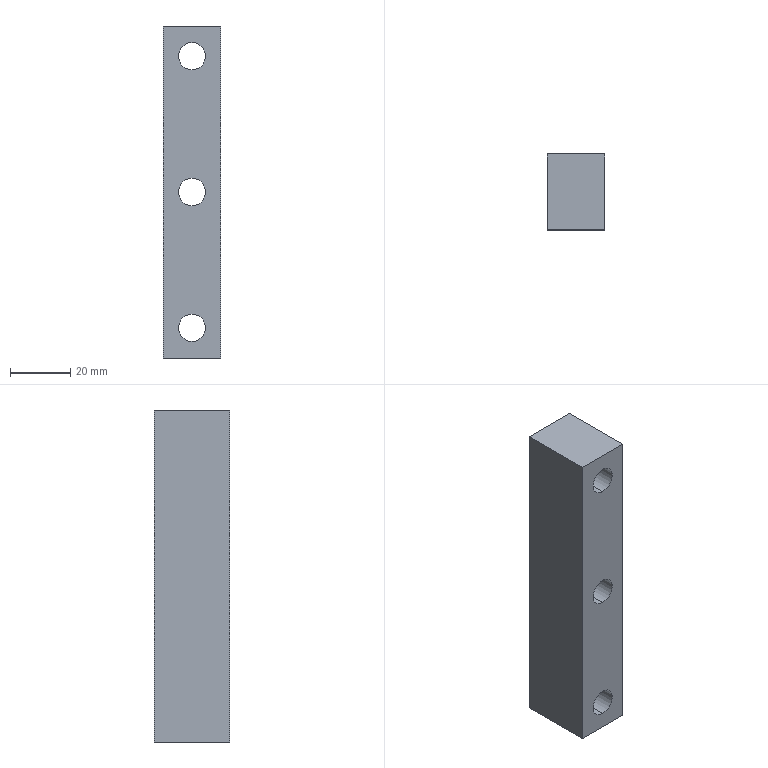Part | STEP file | 0245_214_Block | 1 solid | 29 faces | box 19 x 25 x 110 mm | volume 43111 mm3 | cylinder 16 | plane 9 | cone 4 | commonest cylinder face diameters 9 x6 15 x6 6.8 x4